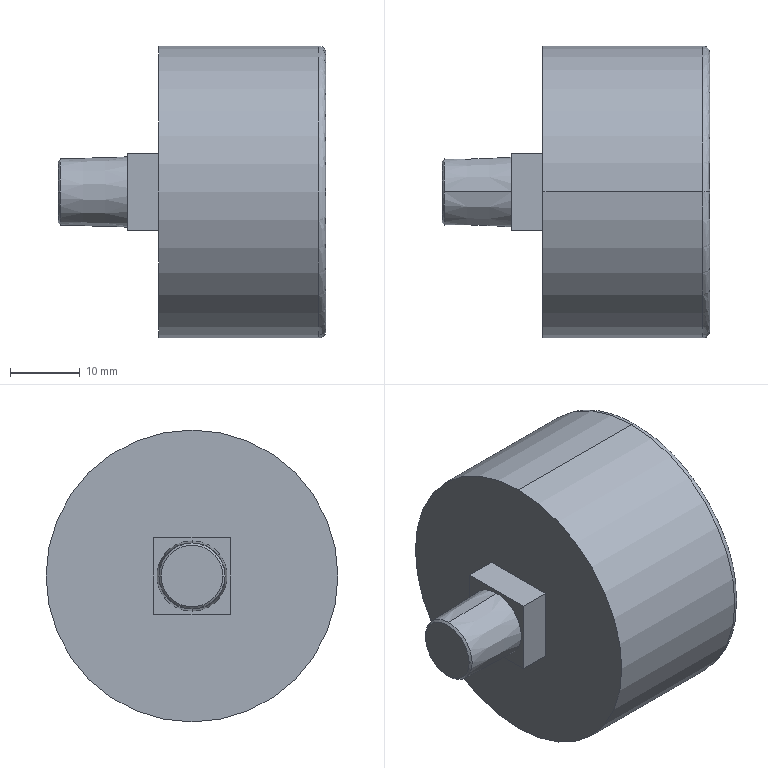Part | STEP file | 1 solid | 18 faces | box 38.5 x 42 x 42 mm | volume 33324 mm3 | plane 8 | cone 6 | cylinder 2 | spline 2 | commonest cylinder face diameters 42 x2
STEP:
#1=CARTESIAN_POINT('',(0.,0.,0.));
#2=DIRECTION('',(0.,0.,1.));
#3=DIRECTION('',(1.,0.,0.));
#4=AXIS2_PLACEMENT_3D('',#1,#2,#3);
#5=CARTESIAN_POINT('',(-38.2,0.,4.748));
#6=VERTEX_POINT('',#5);
#7=CARTESIAN_POINT('',(-38.2,4.748,0.));
#8=VERTEX_POINT('',#7);
#9=CARTESIAN_POINT('',(-38.2,0.,0.));
#10=DIRECTION('',(-1.,0.,0.));
#11=DIRECTION('',(0.,0.,-1.));
#12=AXIS2_PLACEMENT_3D('',#9,#10,#11);
#13=CIRCLE('',#12,4.748);
#14=CARTESIAN_POINT('',(-38.2,0.,0.));
#15=DIRECTION('',(1.,0.,0.));
#16=DIRECTION('',(0.,0.,-1.));
#17=AXIS2_PLACEMENT_3D('',#14,#15,#16);
#18=CONICAL_SURFACE('',#17,4.748,0.03121);
#19=CARTESIAN_POINT('',(6.283,0.));
#20=DIRECTION('',(-1.,0.));
#21=VECTOR('',#20,1.);
#22=LINE('',#19,#21);
#23=(GEOMETRIC_REPRESENTATION_CONTEXT(2)PARAMETRIC_REPRESENTATION_CONTEXT()REPRESENTATION_CONTEXT('',''));
#24=DEFINITIONAL_REPRESENTATION('',(#22),#23);
#25=PCURVE('',#18,#24);
#26=CARTESIAN_POINT('',(-38.5,0.,0.));
#27=DIRECTION('',(1.,0.,0.));
#28=DIRECTION('',(0.,1.,0.));
#29=AXIS2_PLACEMENT_3D('',#26,#27,#28);
#30=CONICAL_SURFACE('',#29,4.439,0.801);
#31=CARTESIAN_POINT('',(4.712,0.2999));
#32=DIRECTION('',(-1.,0.));
#33=VECTOR('',#32,1.);
#34=LINE('',#31,#33);
#35=(GEOMETRIC_REPRESENTATION_CONTEXT(2)PARAMETRIC_REPRESENTATION_CONTEXT()REPRESENTATION_CONTEXT('',''));
#36=DEFINITIONAL_REPRESENTATION('',(#34),#35);
#37=PCURVE('',#30,#36);
#38=SURFACE_CURVE('',#13,(#25,#37),.PCURVE_S1.);
#39=EDGE_CURVE('',#6,#8,#38,.T.);
#40=ORIENTED_EDGE('',*,*,#39,.F.);
#41=CARTESIAN_POINT('',(-28.5,0.,5.051));
#42=VERTEX_POINT('',#41);
#43=CARTESIAN_POINT('',(-38.2,0.,4.748));
#44=DIRECTION('',(0.9995,0.,0.0312));
#45=VECTOR('',#44,1.);
#46=LINE('',#43,#45);
#47=CARTESIAN_POINT('',(3.142,0.));
#48=DIRECTION('',(0.,1.));
#49=VECTOR('',#48,1.);
#50=LINE('',#47,#49);
#51=(GEOMETRIC_REPRESENTATION_CONTEXT(2)PARAMETRIC_REPRESENTATION_CONTEXT()REPRESENTATION_CONTEXT('',''));
#52=DEFINITIONAL_REPRESENTATION('',(#50),#51);
#53=PCURVE('',#18,#52);
#54=CARTESIAN_POINT('',(-38.2,0.,0.));
#55=DIRECTION('',(1.,0.,0.));
#56=DIRECTION('',(0.,0.,-1.));
#57=AXIS2_PLACEMENT_3D('',#54,#55,#56);
#58=CONICAL_SURFACE('',#57,4.748,0.03121);
#59=CARTESIAN_POINT('',(3.142,0.));
#60=DIRECTION('',(0.,1.));
#61=VECTOR('',#60,1.);
#62=LINE('',#59,#61);
#63=(GEOMETRIC_REPRESENTATION_CONTEXT(2)PARAMETRIC_REPRESENTATION_CONTEXT()REPRESENTATION_CONTEXT('',''));
#64=DEFINITIONAL_REPRESENTATION('',(#62),#63);
#65=PCURVE('',#58,#64);
#66=SURFACE_CURVE('',#46,(#53,#65),.PCURVE_S1.);
#67=EDGE_CURVE('',#6,#42,#66,.T.);
#68=ORIENTED_EDGE('',*,*,#67,.T.);
#69=CARTESIAN_POINT('',(-28.5,0.,-5.051));
#70=VERTEX_POINT('',#69);
#71=CARTESIAN_POINT('',(-28.5,0.,0.));
#72=DIRECTION('',(1.,0.,0.));
#73=DIRECTION('',(0.,0.,-1.));
#74=AXIS2_PLACEMENT_3D('',#71,#72,#73);
#75=CIRCLE('',#74,5.051);
#76=CARTESIAN_POINT('',(0.,9.7));
#77=DIRECTION('',(1.,0.));
#78=VECTOR('',#77,1.);
#79=LINE('',#76,#78);
#80=(GEOMETRIC_REPRESENTATION_CONTEXT(2)PARAMETRIC_REPRESENTATION_CONTEXT()REPRESENTATION_CONTEXT('',''));
#81=DEFINITIONAL_REPRESENTATION('',(#79),#80);
#82=PCURVE('',#18,#81);
#83=CARTESIAN_POINT('',(-28.5,-5.5,5.5));
#84=DIRECTION('',(1.,0.,0.));
#85=DIRECTION('',(0.,0.,-1.));
#86=AXIS2_PLACEMENT_3D('',#83,#84,#85);
#87=PLANE('',#86);
#88=CARTESIAN_POINT('',(5.5,5.5));
#89=DIRECTION('',(1.,0.));
#90=AXIS2_PLACEMENT_2D('',#88,#89);
#91=CIRCLE('',#90,5.051);
#92=(GEOMETRIC_REPRESENTATION_CONTEXT(2)PARAMETRIC_REPRESENTATION_CONTEXT()REPRESENTATION_CONTEXT('',''));
#93=DEFINITIONAL_REPRESENTATION('',(#91),#92);
#94=PCURVE('',#87,#93);
#95=SURFACE_CURVE('',#75,(#82,#94),.PCURVE_S1.);
#96=EDGE_CURVE('',#70,#42,#95,.T.);
#97=ORIENTED_EDGE('',*,*,#96,.F.);
#98=CARTESIAN_POINT('',(-38.2,0.,-4.748));
#99=VERTEX_POINT('',#98);
#100=CARTESIAN_POINT('',(-38.2,0.,-4.748));
#101=DIRECTION('',(0.9995,0.,-0.0312));
#102=VECTOR('',#101,1.);
#103=LINE('',#100,#102);
#104=CARTESIAN_POINT('',(0.,0.));
#105=DIRECTION('',(0.,1.));
#106=VECTOR('',#105,1.);
#107=LINE('',#104,#106);
#108=(GEOMETRIC_REPRESENTATION_CONTEXT(2)PARAMETRIC_REPRESENTATION_CONTEXT()REPRESENTATION_CONTEXT('',''));
#109=DEFINITIONAL_REPRESENTATION('',(#107),#108);
#110=PCURVE('',#18,#109);
#111=CARTESIAN_POINT('',(6.283,0.));
#112=DIRECTION('',(0.,1.));
#113=VECTOR('',#112,1.);
#114=LINE('',#111,#113);
#115=(GEOMETRIC_REPRESENTATION_CONTEXT(2)PARAMETRIC_REPRESENTATION_CONTEXT()REPRESENTATION_CONTEXT('',''));
#116=DEFINITIONAL_REPRESENTATION('',(#114),#115);
#117=PCURVE('',#58,#116);
#118=SURFACE_CURVE('',#103,(#110,#117),.PCURVE_S1.);
#119=EDGE_CURVE('',#99,#70,#118,.T.);
#120=ORIENTED_EDGE('',*,*,#119,.F.);
#121=CARTESIAN_POINT('',(-38.2,0.,0.));
#122=DIRECTION('',(-1.,0.,0.));
#123=DIRECTION('',(0.,0.,-1.));
#124=AXIS2_PLACEMENT_3D('',#121,#122,#123);
#125=CIRCLE('',#124,4.748);
#126=CARTESIAN_POINT('',(6.283,0.));
#127=DIRECTION('',(-1.,0.));
#128=VECTOR('',#127,1.);
#129=LINE('',#126,#128);
#130=(GEOMETRIC_REPRESENTATION_CONTEXT(2)PARAMETRIC_REPRESENTATION_CONTEXT()REPRESENTATION_CONTEXT('',''));
#131=DEFINITIONAL_REPRESENTATION('',(#129),#130);
#132=PCURVE('',#18,#131);
#133=CARTESIAN_POINT('',(-38.5,0.,0.));
#134=DIRECTION('',(1.,0.,0.));
#135=DIRECTION('',(0.,1.,0.));
#136=AXIS2_PLACEMENT_3D('',#133,#134,#135);
#137=CONICAL_SURFACE('',#136,4.439,0.801);
#138=CARTESIAN_POINT('',(10.996,0.2999));
#139=DIRECTION('',(-1.,0.));
#140=VECTOR('',#139,1.);
#141=LINE('',#138,#140);
#142=(GEOMETRIC_REPRESENTATION_CONTEXT(2)PARAMETRIC_REPRESENTATION_CONTEXT()REPRESENTATION_CONTEXT('',''));
#143=DEFINITIONAL_REPRESENTATION('',(#141),#142);
#144=PCURVE('',#137,#143);
#145=SURFACE_CURVE('',#125,(#132,#144),.PCURVE_S1.);
#146=EDGE_CURVE('',#8,#99,#145,.T.);
#147=ORIENTED_EDGE('',*,*,#146,.F.);
#148=EDGE_LOOP('',(#40,#68,#97,#120,#147));
#149=FACE_BOUND('',#148,.T.);
#150=ADVANCED_FACE('',(#149),#18,.T.);
#151=CARTESIAN_POINT('',(-38.5,-4.439,0.));
#152=VERTEX_POINT('',#151);
#153=CARTESIAN_POINT('',(-38.5,4.439,0.));
#154=VERTEX_POINT('',#153);
#155=CARTESIAN_POINT('',(-38.5,0.,0.));
#156=DIRECTION('',(-1.,0.,0.));
#157=DIRECTION('',(0.,1.,0.));
#158=AXIS2_PLACEMENT_3D('',#155,#156,#157);
#159=CIRCLE('',#158,4.439);
#160=CARTESIAN_POINT('',(6.283,0.));
#161=DIRECTION('',(-1.,0.));
#162=VECTOR('',#161,1.);
#163=LINE('',#160,#162);
#164=(GEOMETRIC_REPRESENTATION_CONTEXT(2)PARAMETRIC_REPRESENTATION_CONTEXT()REPRESENTATION_CONTEXT('',''));
#165=DEFINITIONAL_REPRESENTATION('',(#163),#164);
#166=PCURVE('',#30,#165);
#167=CARTESIAN_POINT('',(-38.5,-4.492,4.492));
#168=DIRECTION('',(1.,0.,0.));
#169=DIRECTION('',(0.,0.,-1.));
#170=AXIS2_PLACEMENT_3D('',#167,#168,#169);
#171=PLANE('',#170);
#172=CARTESIAN_POINT('',(4.492,8.932));
#173=CARTESIAN_POINT('',(12.181,8.932));
#174=CARTESIAN_POINT('',(8.337,2.273));
#175=CARTESIAN_POINT('',(4.492,-4.386));
#176=CARTESIAN_POINT('',(0.648,2.273));
#177=CARTESIAN_POINT('',(-3.196,8.932));
#178=CARTESIAN_POINT('',(4.492,8.932));
#179=(BOUNDED_CURVE()B_SPLINE_CURVE(2,(#172,#173,#174,#175,#176,#177,#178),.UNSPECIFIED.,.T.,.F.)B_SPLINE_CURVE_WITH_KNOTS((1,2,2,2,2,1),(-2.094,0.,2.094,4.189,6.283,8.378),.UNSPECIFIED.)CURVE()GEOMETRIC_REPRESENTATION_ITEM()RATIONAL_B_SPLINE_CURVE((1.,0.5,1.,0.5,1.,0.5,1.))REPRESENTATION_ITEM(''));
#180=(GEOMETRIC_REPRESENTATION_CONTEXT(2)PARAMETRIC_REPRESENTATION_CONTEXT()REPRESENTATION_CONTEXT('',''));
#181=DEFINITIONAL_REPRESENTATION('',(#179),#180);
#182=PCURVE('',#171,#181);
#183=SURFACE_CURVE('',#159,(#166,#182),.PCURVE_S1.);
#184=EDGE_CURVE('',#152,#154,#183,.T.);
#185=ORIENTED_EDGE('',*,*,#184,.F.);
#186=CARTESIAN_POINT('',(-38.2,-4.748,0.));
#187=VERTEX_POINT('',#186);
#188=CARTESIAN_POINT('',(-38.5,-4.439,0.));
#189=DIRECTION('',(0.696,-0.7181,0.));
#190=VECTOR('',#189,1.);
#191=LINE('',#188,#190);
#192=CARTESIAN_POINT('',(3.142,0.));
#193=DIRECTION('',(0.,1.));
#194=VECTOR('',#193,1.);
#195=LINE('',#192,#194);
#196=(GEOMETRIC_REPRESENTATION_CONTEXT(2)PARAMETRIC_REPRESENTATION_CONTEXT()REPRESENTATION_CONTEXT('',''));
#197=DEFINITIONAL_REPRESENTATION('',(#195),#196);
#198=PCURVE('',#30,#197);
#199=CARTESIAN_POINT('',(3.142,0.));
#200=DIRECTION('',(0.,1.));
#201=VECTOR('',#200,1.);
#202=LINE('',#199,#201);
#203=(GEOMETRIC_REPRESENTATION_CONTEXT(2)PARAMETRIC_REPRESENTATION_CONTEXT()REPRESENTATION_CONTEXT('',''));
#204=DEFINITIONAL_REPRESENTATION('',(#202),#203);
#205=PCURVE('',#137,#204);
#206=SURFACE_CURVE('',#191,(#198,#205),.PCURVE_S1.);
#207=EDGE_CURVE('',#152,#187,#206,.T.);
#208=ORIENTED_EDGE('',*,*,#207,.T.);
#209=CARTESIAN_POINT('',(-38.2,0.,0.));
#210=DIRECTION('',(-1.,0.,0.));
#211=DIRECTION('',(0.,0.,-1.));
#212=AXIS2_PLACEMENT_3D('',#209,#210,#211);
#213=CIRCLE('',#212,4.748);
#214=CARTESIAN_POINT('',(4.712,0.2999));
#215=DIRECTION('',(-1.,0.));
#216=VECTOR('',#215,1.);
#217=LINE('',#214,#216);
#218=(GEOMETRIC_REPRESENTATION_CONTEXT(2)PARAMETRIC_REPRESENTATION_CONTEXT()REPRESENTATION_CONTEXT('',''));
#219=DEFINITIONAL_REPRESENTATION('',(#217),#218);
#220=PCURVE('',#30,#219);
#221=CARTESIAN_POINT('',(6.283,0.));
#222=DIRECTION('',(-1.,0.));
#223=VECTOR('',#222,1.);
#224=LINE('',#221,#223);
#225=(GEOMETRIC_REPRESENTATION_CONTEXT(2)PARAMETRIC_REPRESENTATION_CONTEXT()REPRESENTATION_CONTEXT('',''));
#226=DEFINITIONAL_REPRESENTATION('',(#224),#225);
#227=PCURVE('',#58,#226);
#228=SURFACE_CURVE('',#213,(#220,#227),.PCURVE_S1.);
#229=EDGE_CURVE('',#187,#6,#228,.T.);
#230=ORIENTED_EDGE('',*,*,#229,.T.);
#231=ORIENTED_EDGE('',*,*,#39,.T.);
#232=CARTESIAN_POINT('',(-38.5,4.439,0.));
#233=DIRECTION('',(0.696,0.7181,0.));
#234=VECTOR('',#233,1.);
#235=LINE('',#232,#234);
#236=CARTESIAN_POINT('',(0.,0.));
#237=DIRECTION('',(0.,1.));
#238=VECTOR('',#237,1.);
#239=LINE('',#236,#238);
#240=(GEOMETRIC_REPRESENTATION_CONTEXT(2)PARAMETRIC_REPRESENTATION_CONTEXT()REPRESENTATION_CONTEXT('',''));
#241=DEFINITIONAL_REPRESENTATION('',(#239),#240);
#242=PCURVE('',#30,#241);
#243=CARTESIAN_POINT('',(6.283,0.));
#244=DIRECTION('',(0.,1.));
#245=VECTOR('',#244,1.);
#246=LINE('',#243,#245);
#247=(GEOMETRIC_REPRESENTATION_CONTEXT(2)PARAMETRIC_REPRESENTATION_CONTEXT()REPRESENTATION_CONTEXT('',''));
#248=DEFINITIONAL_REPRESENTATION('',(#246),#247);
#249=PCURVE('',#137,#248);
#250=SURFACE_CURVE('',#235,(#242,#249),.PCURVE_S1.);
#251=EDGE_CURVE('',#154,#8,#250,.T.);
#252=ORIENTED_EDGE('',*,*,#251,.F.);
#253=EDGE_LOOP('',(#185,#208,#230,#231,#252));
#254=FACE_BOUND('',#253,.T.);
#255=ADVANCED_FACE('',(#254),#30,.T.);
#256=CARTESIAN_POINT('',(-24.,0.,-21.));
#257=VERTEX_POINT('',#256);
#258=CARTESIAN_POINT('',(-24.,0.,21.));
#259=VERTEX_POINT('',#258);
#260=CARTESIAN_POINT('',(-24.,0.,0.));
#261=DIRECTION('',(1.,0.,0.));
#262=DIRECTION('',(0.,0.,-1.));
#263=AXIS2_PLACEMENT_3D('',#260,#261,#262);
#264=CIRCLE('',#263,21.);
#265=CARTESIAN_POINT('',(-24.,0.,0.));
#266=DIRECTION('',(1.,0.,0.));
#267=DIRECTION('',(0.,0.,-1.));
#268=AXIS2_PLACEMENT_3D('',#265,#266,#267);
#269=CYLINDRICAL_SURFACE('',#268,21.);
#270=CARTESIAN_POINT('',(0.,0.));
#271=DIRECTION('',(1.,0.));
#272=VECTOR('',#271,1.);
#273=LINE('',#270,#272);
#274=(GEOMETRIC_REPRESENTATION_CONTEXT(2)PARAMETRIC_REPRESENTATION_CONTEXT()REPRESENTATION_CONTEXT('',''));
#275=DEFINITIONAL_REPRESENTATION('',(#273),#274);
#276=PCURVE('',#269,#275);
#277=CARTESIAN_POINT('',(-24.,-21.252,21.252));
#278=DIRECTION('',(1.,0.,0.));
#279=DIRECTION('',(0.,0.,-1.));
#280=AXIS2_PLACEMENT_3D('',#277,#278,#279);
#281=PLANE('',#280);
#282=CARTESIAN_POINT('',(21.252,21.252));
#283=DIRECTION('',(1.,0.));
#284=AXIS2_PLACEMENT_2D('',#282,#283);
#285=CIRCLE('',#284,21.);
#286=(GEOMETRIC_REPRESENTATION_CONTEXT(2)PARAMETRIC_REPRESENTATION_CONTEXT()REPRESENTATION_CONTEXT('',''));
#287=DEFINITIONAL_REPRESENTATION('',(#285),#286);
#288=PCURVE('',#281,#287);
#289=SURFACE_CURVE('',#264,(#276,#288),.PCURVE_S1.);
#290=EDGE_CURVE('',#257,#259,#289,.T.);
#291=ORIENTED_EDGE('',*,*,#290,.T.);
#292=CARTESIAN_POINT('',(-1.,-0.000000006,21.));
#293=VERTEX_POINT('',#292);
#294=CARTESIAN_POINT('',(-24.,0.,21.));
#295=DIRECTION('',(1.,0.,0.));
#296=VECTOR('',#295,1.);
#297=LINE('',#294,#296);
#298=CARTESIAN_POINT('',(3.142,0.));
#299=DIRECTION('',(0.,1.));
#300=VECTOR('',#299,1.);
#301=LINE('',#298,#300);
#302=(GEOMETRIC_REPRESENTATION_CONTEXT(2)PARAMETRIC_REPRESENTATION_CONTEXT()REPRESENTATION_CONTEXT('',''));
#303=DEFINITIONAL_REPRESENTATION('',(#301),#302);
#304=PCURVE('',#269,#303);
#305=CARTESIAN_POINT('',(-24.,0.,0.));
#306=DIRECTION('',(1.,0.,0.));
#307=DIRECTION('',(0.,0.,-1.));
#308=AXIS2_PLACEMENT_3D('',#305,#306,#307);
#309=CYLINDRICAL_SURFACE('',#308,21.);
#310=CARTESIAN_POINT('',(3.142,0.));
#311=DIRECTION('',(0.,1.));
#312=VECTOR('',#311,1.);
#313=LINE('',#310,#312);
#314=(GEOMETRIC_REPRESENTATION_CONTEXT(2)PARAMETRIC_REPRESENTATION_CONTEXT()REPRESENTATION_CONTEXT('',''));
#315=DEFINITIONAL_REPRESENTATION('',(#313),#314);
#316=PCURVE('',#309,#315);
#317=SURFACE_CURVE('',#297,(#304,#316),.PCURVE_S1.);
#318=EDGE_CURVE('',#259,#293,#317,.T.);
#319=ORIENTED_EDGE('',*,*,#318,.T.);
#320=CARTESIAN_POINT('',(-1.,-0.000000001,-21.));
#321=VERTEX_POINT('',#320);
#322=CARTESIAN_POINT('',(-1.,0.,0.));
#323=DIRECTION('',(1.,0.,0.));
#324=DIRECTION('',(0.,0.,-1.));
#325=AXIS2_PLACEMENT_3D('',#322,#323,#324);
#326=CIRCLE('',#325,21.);
#327=CARTESIAN_POINT('',(0.,23.));
#328=DIRECTION('',(1.,0.));
#329=VECTOR('',#328,1.);
#330=LINE('',#327,#329);
#331=(GEOMETRIC_REPRESENTATION_CONTEXT(2)PARAMETRIC_REPRESENTATION_CONTEXT()REPRESENTATION_CONTEXT('',''));
#332=DEFINITIONAL_REPRESENTATION('',(#330),#331);
#333=PCURVE('',#269,#332);
#334=CARTESIAN_POINT('',(-0.004996,0.,-19.9));
#335=CARTESIAN_POINT('',(-0.004996,39.8,-19.9));
#336=CARTESIAN_POINT('',(-0.004996,39.8,19.9));
#337=CARTESIAN_POINT('',(-0.004996,0.,19.9));
#338=CARTESIAN_POINT('',(0.06322,0.,-20.58));
#339=CARTESIAN_POINT('',(0.06322,41.16,-20.58));
#340=CARTESIAN_POINT('',(0.06322,41.16,20.58));
#341=CARTESIAN_POINT('',(0.06322,0.,20.58));
#342=CARTESIAN_POINT('',(-0.4199,0.,-21.063));
#343=CARTESIAN_POINT('',(-0.4199,42.126,-21.063));
#344=CARTESIAN_POINT('',(-0.4199,42.126,21.063));
#345=CARTESIAN_POINT('',(-0.4199,0.,21.063));
#346=CARTESIAN_POINT('',(-1.1,0.,-20.995));
#347=CARTESIAN_POINT('',(-1.1,41.99,-20.995));
#348=CARTESIAN_POINT('',(-1.1,41.99,20.995));
#349=CARTESIAN_POINT('',(-1.1,0.,20.995));
#350=(BOUNDED_SURFACE()B_SPLINE_SURFACE(3,3,((#334,#335,#336,#337),(#338,#339,#340,#341),(#342,#343,#344,#345),(#346,#347,#348,#349)),.UNSPECIFIED.,.F.,.F.,.F.)B_SPLINE_SURFACE_WITH_KNOTS((4,4),(4,4),(0.,1.),(0.,1.),.PIECEWISE_BEZIER_KNOTS.)GEOMETRIC_REPRESENTATION_ITEM()RATIONAL_B_SPLINE_SURFACE(((1.,0.3333,0.3333,1.),(0.7553,0.2518,0.2518,0.7553),(0.7553,0.2518,0.2518,0.7553),(1.,0.3333,0.3333,1.)))REPRESENTATION_ITEM('')SURFACE());
#351=CARTESIAN_POINT('',(0.9369,0.));
#352=CARTESIAN_POINT('',(0.9369,0.02375));
#353=CARTESIAN_POINT('',(0.9369,0.06805));
#354=CARTESIAN_POINT('',(0.9369,0.1267));
#355=CARTESIAN_POINT('',(0.9369,0.1794));
#356=CARTESIAN_POINT('',(0.9369,0.2276));
#357=CARTESIAN_POINT('',(0.9369,0.2721));
#358=CARTESIAN_POINT('',(0.9369,0.3139));
#359=CARTESIAN_POINT('',(0.9369,0.3535));
#360=CARTESIAN_POINT('',(0.9369,0.3914));
#361=CARTESIAN_POINT('',(0.9369,0.4282));
#362=CARTESIAN_POINT('',(0.9369,0.4643));
#363=CARTESIAN_POINT('',(0.9369,0.5));
#364=CARTESIAN_POINT('',(0.9369,0.5357));
#365=CARTESIAN_POINT('',(0.9369,0.5718));
#366=CARTESIAN_POINT('',(0.9369,0.6086));
#367=CARTESIAN_POINT('',(0.9369,0.6465));
#368=CARTESIAN_POINT('',(0.9369,0.6861));
#369=CARTESIAN_POINT('',(0.9369,0.7279));
#370=CARTESIAN_POINT('',(0.9369,0.7724));
#371=CARTESIAN_POINT('',(0.9369,0.8206));
#372=CARTESIAN_POINT('',(0.9369,0.8733));
#373=CARTESIAN_POINT('',(0.9369,0.9319));
#374=CARTESIAN_POINT('',(0.9369,0.9763));
#375=CARTESIAN_POINT('',(0.9369,1.));
#376=B_SPLINE_CURVE_WITH_KNOTS('',3,(#351,#352,#353,#354,#355,#356,#357,#358,#359,#360,#361,#362,#363,#364,#365,#366,#367,#368,#369,#370,#371,#372,#373,#374,#375),.UNSPECIFIED.,.F.,.F.,(4,1,1,1,1,1,1,1,1,1,1,1,1,1,1,1,1,1,1,1,1,1,4),(0.,0.1428,0.2856,0.4284,0.5712,0.714,0.8568,0.9996,1.142,1.285,1.428,1.571,1.714,1.856,1.999,2.142,2.285,2.428,2.57,2.713,2.856,2.999,3.142),.QUASI_UNIFORM_KNOTS.);
#377=(GEOMETRIC_REPRESENTATION_CONTEXT(2)PARAMETRIC_REPRESENTATION_CONTEXT()REPRESENTATION_CONTEXT('',''));
#378=DEFINITIONAL_REPRESENTATION('',(#376),#377);
#379=PCURVE('',#350,#378);
#380=SURFACE_CURVE('',#326,(#333,#379),.PCURVE_S1.);
#381=EDGE_CURVE('',#321,#293,#380,.T.);
#382=ORIENTED_EDGE('',*,*,#381,.F.);
#383=CARTESIAN_POINT('',(-24.,0.,-21.));
#384=DIRECTION('',(1.,0.,0.));
#385=VECTOR('',#384,1.);
#386=LINE('',#383,#385);
#387=CARTESIAN_POINT('',(0.,0.));
#388=DIRECTION('',(0.,1.));
#389=VECTOR('',#388,1.);
#390=LINE('',#387,#389);
#391=(GEOMETRIC_REPRESENTATION_CONTEXT(2)PARAMETRIC_REPRESENTATION_CONTEXT()REPRESENTATION_CONTEXT('',''));
#392=DEFINITIONAL_REPRESENTATION('',(#390),#391);
#393=PCURVE('',#269,#392);
#394=CARTESIAN_POINT('',(6.283,0.));
#395=DIRECTION('',(0.,1.));
#396=VECTOR('',#395,1.);
#397=LINE('',#394,#396);
#398=(GEOMETRIC_REPRESENTATION_CONTEXT(2)PARAMETRIC_REPRESENTATION_CONTEXT()REPRESENTATION_CONTEXT('',''));
#399=DEFINITIONAL_REPRESENTATION('',(#397),#398);
#400=PCURVE('',#309,#399);
#401=SURFACE_CURVE('',#386,(#393,#400),.PCURVE_S1.);
#402=EDGE_CURVE('',#257,#321,#401,.T.);
#403=ORIENTED_EDGE('',*,*,#402,.F.);
#404=EDGE_LOOP('',(#291,#319,#382,#403));
#405=FACE_BOUND('',#404,.T.);
#406=ADVANCED_FACE('',(#405),#269,.T.);
#407=CARTESIAN_POINT('',(-1.,0.,-19.));
#408=VERTEX_POINT('',#407);
#409=CARTESIAN_POINT('',(0.,0.,-20.));
#410=VERTEX_POINT('',#409);
#411=CARTESIAN_POINT('',(-1.,0.,-19.));
#412=DIRECTION('',(0.7071,0.,-0.7071));
#413=VECTOR('',#412,1.);
#414=LINE('',#411,#413);
#415=CARTESIAN_POINT('',(-1.,0.,0.));
#416=DIRECTION('',(1.,0.,0.));
#417=DIRECTION('',(0.,0.,-1.));
#418=AXIS2_PLACEMENT_3D('',#415,#416,#417);
#419=CONICAL_SURFACE('',#418,19.,0.7854);
#420=CARTESIAN_POINT('',(6.283,0.));
#421=DIRECTION('',(0.,1.));
#422=VECTOR('',#421,1.);
#423=LINE('',#420,#422);
#424=(GEOMETRIC_REPRESENTATION_CONTEXT(2)PARAMETRIC_REPRESENTATION_CONTEXT()REPRESENTATION_CONTEXT('',''));
#425=DEFINITIONAL_REPRESENTATION('',(#423),#424);
#426=PCURVE('',#419,#425);
#427=CARTESIAN_POINT('',(-1.,0.,0.));
#428=DIRECTION('',(1.,0.,0.));
#429=DIRECTION('',(0.,0.,-1.));
#430=AXIS2_PLACEMENT_3D('',#427,#428,#429);
#431=CONICAL_SURFACE('',#430,19.,0.7854);
#432=CARTESIAN_POINT('',(0.,0.));
#433=DIRECTION('',(0.,1.));
#434=VECTOR('',#433,1.);
#435=LINE('',#432,#434);
#436=(GEOMETRIC_REPRESENTATION_CONTEXT(2)PARAMETRIC_REPRESENTATION_CONTEXT()REPRESENTATION_CONTEXT('',''));
#437=DEFINITIONAL_REPRESENTATION('',(#435),#436);
#438=PCURVE('',#431,#437);
#439=SURFACE_CURVE('',#414,(#426,#438),.PCURVE_S1.);
#440=EDGE_CURVE('',#408,#410,#439,.T.);
#441=ORIENTED_EDGE('',*,*,#440,.T.);
#442=CARTESIAN_POINT('',(0.,-0.000000002,20.));
#443=VERTEX_POINT('',#442);
#444=CARTESIAN_POINT('',(0.,0.,0.));
#445=DIRECTION('',(-1.,0.,0.));
#446=DIRECTION('',(0.,-1.,0.));
#447=AXIS2_PLACEMENT_3D('',#444,#445,#446);
#448=CIRCLE('',#447,20.);
#449=CARTESIAN_POINT('',(10.996,1.));
#450=DIRECTION('',(-1.,0.));
#451=VECTOR('',#450,1.);
#452=LINE('',#449,#451);
#453=(GEOMETRIC_REPRESENTATION_CONTEXT(2)PARAMETRIC_REPRESENTATION_CONTEXT()REPRESENTATION_CONTEXT('',''));
#454=DEFINITIONAL_REPRESENTATION('',(#452),#453);
#455=PCURVE('',#419,#454);
#456=CARTESIAN_POINT('',(-0.004996,0.,19.9));
#457=CARTESIAN_POINT('',(-0.004996,-39.8,19.9));
#458=CARTESIAN_POINT('',(-0.004996,-39.8,-19.9));
#459=CARTESIAN_POINT('',(-0.004996,0.,-19.9));
#460=CARTESIAN_POINT('',(0.06322,0.,20.58));
#461=CARTESIAN_POINT('',(0.06322,-41.16,20.58));
#462=CARTESIAN_POINT('',(0.06322,-41.16,-20.58));
#463=CARTESIAN_POINT('',(0.06322,0.,-20.58));
#464=CARTESIAN_POINT('',(-0.4199,0.,21.063));
#465=CARTESIAN_POINT('',(-0.4199,-42.126,21.063));
#466=CARTESIAN_POINT('',(-0.4199,-42.126,-21.063));
#467=CARTESIAN_POINT('',(-0.4199,0.,-21.063));
#468=CARTESIAN_POINT('',(-1.1,0.,20.995));
#469=CARTESIAN_POINT('',(-1.1,-41.99,20.995));
#470=CARTESIAN_POINT('',(-1.1,-41.99,-20.995));
#471=CARTESIAN_POINT('',(-1.1,0.,-20.995));
#472=(BOUNDED_SURFACE()B_SPLINE_SURFACE(3,3,((#456,#457,#458,#459),(#460,#461,#462,#463),(#464,#465,#466,#467),(#468,#469,#470,#471)),.UNSPECIFIED.,.F.,.F.,.F.)B_SPLINE_SURFACE_WITH_KNOTS((4,4),(4,4),(0.,1.),(0.,1.),.PIECEWISE_BEZIER_KNOTS.)GEOMETRIC_REPRESENTATION_ITEM()RATIONAL_B_SPLINE_SURFACE(((1.,0.3333,0.3333,1.),(0.7553,0.2518,0.2518,0.7553),(0.7553,0.2518,0.2518,0.7553),(1.,0.3333,0.3333,1.)))REPRESENTATION_ITEM('')SURFACE());
#473=CARTESIAN_POINT('',(0.06314,1.));
#474=CARTESIAN_POINT('',(0.06314,0.9763));
#475=CARTESIAN_POINT('',(0.06314,0.9319));
#476=CARTESIAN_POINT('',(0.06314,0.8733));
#477=CARTESIAN_POINT('',(0.06314,0.8206));
#478=CARTESIAN_POINT('',(0.06314,0.7724));
#479=CARTESIAN_POINT('',(0.06314,0.7279));
#480=CARTESIAN_POINT('',(0.06314,0.6861));
#481=CARTESIAN_POINT('',(0.06314,0.6465));
#482=CARTESIAN_POINT('',(0.06314,0.6086));
#483=CARTESIAN_POINT('',(0.06314,0.5718));
#484=CARTESIAN_POINT('',(0.06314,0.5357));
#485=CARTESIAN_POINT('',(0.06314,0.5));
#486=CARTESIAN_POINT('',(0.06314,0.4643));
#487=CARTESIAN_POINT('',(0.06314,0.4282));
#488=CARTESIAN_POINT('',(0.06314,0.3914));
#489=CARTESIAN_POINT('',(0.06314,0.3535));
#490=CARTESIAN_POINT('',(0.06314,0.3139));
#491=CARTESIAN_POINT('',(0.06314,0.2721));
#492=CARTESIAN_POINT('',(0.06314,0.2276));
#493=CARTESIAN_POINT('',(0.06314,0.1794));
#494=CARTESIAN_POINT('',(0.06314,0.1267));
#495=CARTESIAN_POINT('',(0.06314,0.06805));
#496=CARTESIAN_POINT('',(0.06314,0.02375));
#497=CARTESIAN_POINT('',(0.06314,0.));
#498=B_SPLINE_CURVE_WITH_KNOTS('',3,(#473,#474,#475,#476,#477,#478,#479,#480,#481,#482,#483,#484,#485,#486,#487,#488,#489,#490,#491,#492,#493,#494,#495,#496,#497),.UNSPECIFIED.,.F.,.F.,(4,1,1,1,1,1,1,1,1,1,1,1,1,1,1,1,1,1,1,1,1,1,4),(4.712,4.855,4.998,5.141,5.284,5.426,5.569,5.712,5.855,5.998,6.14,6.283,6.426,6.569,6.712,6.854,6.997,7.14,7.283,7.426,7.568,7.711,7.854),.QUASI_UNIFORM_KNOTS.);
#499=(GEOMETRIC_REPRESENTATION_CONTEXT(2)PARAMETRIC_REPRESENTATION_CONTEXT()REPRESENTATION_CONTEXT('',''));
#500=DEFINITIONAL_REPRESENTATION('',(#498),#499);
#501=PCURVE('',#472,#500);
#502=SURFACE_CURVE('',#448,(#455,#501),.PCURVE_S1.);
#503=EDGE_CURVE('',#410,#443,#502,.T.);
#504=ORIENTED_EDGE('',*,*,#503,.T.);
#505=CARTESIAN_POINT('',(-1.,0.,19.));
#506=VERTEX_POINT('',#505);
#507=CARTESIAN_POINT('',(-1.,0.,19.));
#508=DIRECTION('',(0.7071,0.,0.7071));
#509=VECTOR('',#508,1.);
#510=LINE('',#507,#509);
#511=CARTESIAN_POINT('',(3.142,0.));
#512=DIRECTION('',(0.,1.));
#513=VECTOR('',#512,1.);
#514=LINE('',#511,#513);
#515=(GEOMETRIC_REPRESENTATION_CONTEXT(2)PARAMETRIC_REPRESENTATION_CONTEXT()REPRESENTATION_CONTEXT('',''));
#516=DEFINITIONAL_REPRESENTATION('',(#514),#515);
#517=PCURVE('',#419,#516);
#518=CARTESIAN_POINT('',(3.142,0.));
#519=DIRECTION('',(0.,1.));
#520=VECTOR('',#519,1.);
#521=LINE('',#518,#520);
#522=(GEOMETRIC_REPRESENTATION_CONTEXT(2)PARAMETRIC_REPRESENTATION_CONTEXT()REPRESENTATION_CONTEXT('',''));
#523=DEFINITIONAL_REPRESENTATION('',(#521),#522);
#524=PCURVE('',#431,#523);
#525=SURFACE_CURVE('',#510,(#517,#524),.PCURVE_S1.);
#526=EDGE_CURVE('',#506,#443,#525,.T.);
#527=ORIENTED_EDGE('',*,*,#526,.F.);
#528=CARTESIAN_POINT('',(-1.,0.,0.));
#529=DIRECTION('',(-1.,0.,0.));
#530=DIRECTION('',(0.,0.,-1.));
#531=AXIS2_PLACEMENT_3D('',#528,#529,#530);
#532=CIRCLE('',#531,19.);
#533=CARTESIAN_POINT('',(6.283,0.));
#534=DIRECTION('',(-1.,0.));
#535=VECTOR('',#534,1.);
#536=LINE('',#533,#535);
#537=(GEOMETRIC_REPRESENTATION_CONTEXT(2)PARAMETRIC_REPRESENTATION_CONTEXT()REPRESENTATION_CONTEXT('',''));
#538=DEFINITIONAL_REPRESENTATION('',(#536),#537);
#539=PCURVE('',#419,#538);
#540=CARTESIAN_POINT('',(-1.,-19.228,-19.228));
#541=DIRECTION('',(-1.,0.,0.));
#542=DIRECTION('',(0.,0.,1.));
#543=AXIS2_PLACEMENT_3D('',#540,#541,#542);
#544=PLANE('',#543);
#545=CARTESIAN_POINT('',(19.228,19.228));
#546=DIRECTION('',(-1.,0.));
#547=AXIS2_PLACEMENT_2D('',#545,#546);
#548=CIRCLE('',#547,19.);
#549=(GEOMETRIC_REPRESENTATION_CONTEXT(2)PARAMETRIC_REPRESENTATION_CONTEXT()REPRESENTATION_CONTEXT('',''));
#550=DEFINITIONAL_REPRESENTATION('',(#548),#549);
#551=PCURVE('',#544,#550);
#552=SURFACE_CURVE('',#532,(#539,#551),.PCURVE_S1.);
#553=EDGE_CURVE('',#408,#506,#552,.T.);
#554=ORIENTED_EDGE('',*,*,#553,.F.);
#555=EDGE_LOOP('',(#441,#504,#527,#554));
#556=FACE_BOUND('',#555,.F.);
#557=ADVANCED_FACE('',(#556),#419,.F.);
#558=ORIENTED_EDGE('',*,*,#67,.F.);
#559=ORIENTED_EDGE('',*,*,#229,.F.);
#560=CARTESIAN_POINT('',(-38.2,0.,0.));
#561=DIRECTION('',(-1.,0.,0.));
#562=DIRECTION('',(0.,0.,-1.));
#563=AXIS2_PLACEMENT_3D('',#560,#561,#562);
#564=CIRCLE('',#563,4.748);
#565=CARTESIAN_POINT('',(6.283,0.));
#566=DIRECTION('',(-1.,0.));
#567=VECTOR('',#566,1.);
#568=LINE('',#565,#567);
#569=(GEOMETRIC_REPRESENTATION_CONTEXT(2)PARAMETRIC_REPRESENTATION_CONTEXT()REPRESENTATION_CONTEXT('',''));
#570=DEFINITIONAL_REPRESENTATION('',(#568),#569);
#571=PCURVE('',#58,#570);
#572=CARTESIAN_POINT('',(4.712,0.2999));
#573=DIRECTION('',(-1.,0.));
#574=VECTOR('',#573,1.);
#575=LINE('',#572,#574);
#576=(GEOMETRIC_REPRESENTATION_CONTEXT(2)PARAMETRIC_REPRESENTATION_CONTEXT()REPRESENTATION_CONTEXT('',''));
#577=DEFINITIONAL_REPRESENTATION('',(#575),#576);
#578=PCURVE('',#137,#577);
#579=SURFACE_CURVE('',#564,(#571,#578),.PCURVE_S1.);
#580=EDGE_CURVE('',#99,#187,#579,.T.);
#581=ORIENTED_EDGE('',*,*,#580,.F.);
#582=ORIENTED_EDGE('',*,*,#119,.T.);
#583=CARTESIAN_POINT('',(-28.5,0.,0.));
#584=DIRECTION('',(1.,0.,0.));
#585=DIRECTION('',(0.,0.,-1.));
#586=AXIS2_PLACEMENT_3D('',#583,#584,#585);
#587=CIRCLE('',#586,5.051);
#588=CARTESIAN_POINT('',(0.,9.7));
#589=DIRECTION('',(1.,0.));
#590=VECTOR('',#589,1.);
#591=LINE('',#588,#590);
#592=(GEOMETRIC_REPRESENTATION_CONTEXT(2)PARAMETRIC_REPRESENTATION_CONTEXT()REPRESENTATION_CONTEXT('',''));
#593=DEFINITIONAL_REPRESENTATION('',(#591),#592);
#594=PCURVE('',#58,#593);
#595=CARTESIAN_POINT('',(5.5,5.5));
#596=DIRECTION('',(1.,0.));
#597=AXIS2_PLACEMENT_2D('',#595,#596);
#598=CIRCLE('',#597,5.051);
#599=(GEOMETRIC_REPRESENTATION_CONTEXT(2)PARAMETRIC_REPRESENTATION_CONTEXT()REPRESENTATION_CONTEXT('',''));
#600=DEFINITIONAL_REPRESENTATION('',(#598),#599);
#601=PCURVE('',#87,#600);
#602=SURFACE_CURVE('',#587,(#594,#601),.PCURVE_S1.);
#603=EDGE_CURVE('',#42,#70,#602,.T.);
#604=ORIENTED_EDGE('',*,*,#603,.F.);
#605=EDGE_LOOP('',(#558,#559,#581,#582,#604));
#606=FACE_BOUND('',#605,.T.);
#607=ADVANCED_FACE('',(#606),#58,.T.);
#608=ORIENTED_EDGE('',*,*,#207,.F.);
#609=CARTESIAN_POINT('',(-38.5,0.,0.));
#610=DIRECTION('',(-1.,0.,0.));
#611=DIRECTION('',(0.,1.,0.));
#612=AXIS2_PLACEMENT_3D('',#609,#610,#611);
#613=CIRCLE('',#612,4.439);
#614=CARTESIAN_POINT('',(6.283,0.));
#615=DIRECTION('',(-1.,0.));
#616=VECTOR('',#615,1.);
#617=LINE('',#614,#616);
#618=(GEOMETRIC_REPRESENTATION_CONTEXT(2)PARAMETRIC_REPRESENTATION_CONTEXT()REPRESENTATION_CONTEXT('',''));
#619=DEFINITIONAL_REPRESENTATION('',(#617),#618);
#620=PCURVE('',#137,#619);
#621=CARTESIAN_POINT('',(4.492,8.932));
#622=CARTESIAN_POINT('',(12.181,8.932));
#623=CARTESIAN_POINT('',(8.337,2.273));
#624=CARTESIAN_POINT('',(4.492,-4.386));
#625=CARTESIAN_POINT('',(0.648,2.273));
#626=CARTESIAN_POINT('',(-3.196,8.932));
#627=CARTESIAN_POINT('',(4.492,8.932));
#628=(BOUNDED_CURVE()B_SPLINE_CURVE(2,(#621,#622,#623,#624,#625,#626,#627),.UNSPECIFIED.,.T.,.F.)B_SPLINE_CURVE_WITH_KNOTS((1,2,2,2,2,1),(-2.094,0.,2.094,4.189,6.283,8.378),.UNSPECIFIED.)CURVE()GEOMETRIC_REPRESENTATION_ITEM()RATIONAL_B_SPLINE_CURVE((1.,0.5,1.,0.5,1.,0.5,1.))REPRESENTATION_ITEM(''));
#629=(GEOMETRIC_REPRESENTATION_CONTEXT(2)PARAMETRIC_REPRESENTATION_CONTEXT()REPRESENTATION_CONTEXT('',''));
#630=DEFINITIONAL_REPRESENTATION('',(#628),#629);
#631=PCURVE('',#171,#630);
#632=SURFACE_CURVE('',#613,(#620,#631),.PCURVE_S1.);
#633=EDGE_CURVE('',#154,#152,#632,.T.);
#634=ORIENTED_EDGE('',*,*,#633,.F.);
#635=ORIENTED_EDGE('',*,*,#251,.T.);
#636=ORIENTED_EDGE('',*,*,#146,.T.);
#637=ORIENTED_EDGE('',*,*,#580,.T.);
#638=EDGE_LOOP('',(#608,#634,#635,#636,#637));
#639=FACE_BOUND('',#638,.T.);
#640=ADVANCED_FACE('',(#639),#137,.T.);
#641=ORIENTED_EDGE('',*,*,#96,.T.);
#642=ORIENTED_EDGE('',*,*,#603,.T.);
#643=EDGE_LOOP('',(#641,#642));
#644=FACE_BOUND('',#643,.T.);
#645=CARTESIAN_POINT('',(-28.5,-5.5,-5.5));
#646=VERTEX_POINT('',#645);
#647=CARTESIAN_POINT('',(-28.5,5.5,-5.5));
#648=VERTEX_POINT('',#647);
#649=CARTESIAN_POINT('',(-28.5,0.,-5.5));
#650=DIRECTION('',(0.,1.,0.));
#651=VECTOR('',#650,1.);
#652=LINE('',#649,#651);
#653=CARTESIAN_POINT('',(11.,5.5));
#654=DIRECTION('',(0.,1.));
#655=VECTOR('',#654,1.);
#656=LINE('',#653,#655);
#657=(GEOMETRIC_REPRESENTATION_CONTEXT(2)PARAMETRIC_REPRESENTATION_CONTEXT()REPRESENTATION_CONTEXT('',''));
#658=DEFINITIONAL_REPRESENTATION('',(#656),#657);
#659=PCURVE('',#87,#658);
#660=CARTESIAN_POINT('',(-24.,-5.5,-5.5));
#661=DIRECTION('',(0.,0.,-1.));
#662=DIRECTION('',(-1.,0.,0.));
#663=AXIS2_PLACEMENT_3D('',#660,#661,#662);
#664=PLANE('',#663);
#665=CARTESIAN_POINT('',(4.5,5.5));
#666=DIRECTION('',(0.,1.));
#667=VECTOR('',#666,1.);
#668=LINE('',#665,#667);
#669=(GEOMETRIC_REPRESENTATION_CONTEXT(2)PARAMETRIC_REPRESENTATION_CONTEXT()REPRESENTATION_CONTEXT('',''));
#670=DEFINITIONAL_REPRESENTATION('',(#668),#669);
#671=PCURVE('',#664,#670);
#672=SURFACE_CURVE('',#652,(#659,#671),.PCURVE_S1.);
#673=EDGE_CURVE('',#646,#648,#672,.T.);
#674=ORIENTED_EDGE('',*,*,#673,.F.);
#675=CARTESIAN_POINT('',(-28.5,-5.5,5.5));
#676=VERTEX_POINT('',#675);
#677=CARTESIAN_POINT('',(-28.5,-5.5,0.));
#678=DIRECTION('',(0.,0.,-1.));
#679=VECTOR('',#678,1.);
#680=LINE('',#677,#679);
#681=CARTESIAN_POINT('',(5.5,0.));
#682=DIRECTION('',(1.,0.));
#683=VECTOR('',#682,1.);
#684=LINE('',#681,#683);
#685=(GEOMETRIC_REPRESENTATION_CONTEXT(2)PARAMETRIC_REPRESENTATION_CONTEXT()REPRESENTATION_CONTEXT('',''));
#686=DEFINITIONAL_REPRESENTATION('',(#684),#685);
#687=PCURVE('',#87,#686);
#688=CARTESIAN_POINT('',(-28.5,-5.5,5.5));
#689=DIRECTION('',(0.,-1.,0.));
#690=DIRECTION('',(0.,0.,-1.));
#691=AXIS2_PLACEMENT_3D('',#688,#689,#690);
#692=PLANE('',#691);
#693=CARTESIAN_POINT('',(5.5,0.));
#694=DIRECTION('',(1.,0.));
#695=VECTOR('',#694,1.);
#696=LINE('',#693,#695);
#697=(GEOMETRIC_REPRESENTATION_CONTEXT(2)PARAMETRIC_REPRESENTATION_CONTEXT()REPRESENTATION_CONTEXT('',''));
#698=DEFINITIONAL_REPRESENTATION('',(#696),#697);
#699=PCURVE('',#692,#698);
#700=SURFACE_CURVE('',#680,(#687,#699),.PCURVE_S1.);
#701=EDGE_CURVE('',#676,#646,#700,.T.);
#702=ORIENTED_EDGE('',*,*,#701,.F.);
#703=CARTESIAN_POINT('',(-28.5,5.5,5.5));
#704=VERTEX_POINT('',#703);
#705=CARTESIAN_POINT('',(-28.5,0.,5.5));
#706=DIRECTION('',(0.,-1.,0.));
#707=VECTOR('',#706,1.);
#708=LINE('',#705,#707);
#709=CARTESIAN_POINT('',(0.,5.5));
#710=DIRECTION('',(0.,-1.));
#711=VECTOR('',#710,1.);
#712=LINE('',#709,#711);
#713=(GEOMETRIC_REPRESENTATION_CONTEXT(2)PARAMETRIC_REPRESENTATION_CONTEXT()REPRESENTATION_CONTEXT('',''));
#714=DEFINITIONAL_REPRESENTATION('',(#712),#713);
#715=PCURVE('',#87,#714);
#716=CARTESIAN_POINT('',(-28.5,-5.5,5.5));
#717=DIRECTION('',(0.,0.,1.));
#718=DIRECTION('',(1.,0.,0.));
#719=AXIS2_PLACEMENT_3D('',#716,#717,#718);
#720=PLANE('',#719);
#721=CARTESIAN_POINT('',(0.,5.5));
#722=DIRECTION('',(0.,-1.));
#723=VECTOR('',#722,1.);
#724=LINE('',#721,#723);
#725=(GEOMETRIC_REPRESENTATION_CONTEXT(2)PARAMETRIC_REPRESENTATION_CONTEXT()REPRESENTATION_CONTEXT('',''));
#726=DEFINITIONAL_REPRESENTATION('',(#724),#725);
#727=PCURVE('',#720,#726);
#728=SURFACE_CURVE('',#708,(#715,#727),.PCURVE_S1.);
#729=EDGE_CURVE('',#704,#676,#728,.T.);
#730=ORIENTED_EDGE('',*,*,#729,.F.);
#731=CARTESIAN_POINT('',(-28.5,5.5,0.));
#732=DIRECTION('',(0.,0.,1.));
#733=VECTOR('',#732,1.);
#734=LINE('',#731,#733);
#735=CARTESIAN_POINT('',(5.5,11.));
#736=DIRECTION('',(-1.,0.));
#737=VECTOR('',#736,1.);
#738=LINE('',#735,#737);
#739=(GEOMETRIC_REPRESENTATION_CONTEXT(2)PARAMETRIC_REPRESENTATION_CONTEXT()REPRESENTATION_CONTEXT('',''));
#740=DEFINITIONAL_REPRESENTATION('',(#738),#739);
#741=PCURVE('',#87,#740);
#742=CARTESIAN_POINT('',(-28.5,5.5,-5.5));
#743=DIRECTION('',(0.,1.,0.));
#744=DIRECTION('',(0.,0.,1.));
#745=AXIS2_PLACEMENT_3D('',#742,#743,#744);
#746=PLANE('',#745);
#747=CARTESIAN_POINT('',(5.5,0.));
#748=DIRECTION('',(1.,0.));
#749=VECTOR('',#748,1.);
#750=LINE('',#747,#749);
#751=(GEOMETRIC_REPRESENTATION_CONTEXT(2)PARAMETRIC_REPRESENTATION_CONTEXT()REPRESENTATION_CONTEXT('',''));
#752=DEFINITIONAL_REPRESENTATION('',(#750),#751);
#753=PCURVE('',#746,#752);
#754=SURFACE_CURVE('',#734,(#741,#753),.PCURVE_S1.);
#755=EDGE_CURVE('',#648,#704,#754,.T.);
#756=ORIENTED_EDGE('',*,*,#755,.F.);
#757=EDGE_LOOP('',(#674,#702,#730,#756));
#758=FACE_BOUND('',#757,.T.);
#759=ADVANCED_FACE('',(#644,#758),#87,.F.);
#760=ORIENTED_EDGE('',*,*,#633,.T.);
#761=ORIENTED_EDGE('',*,*,#184,.T.);
#762=EDGE_LOOP('',(#760,#761));
#763=FACE_BOUND('',#762,.T.);
#764=ADVANCED_FACE('',(#763),#171,.F.);
#765=CARTESIAN_POINT('',(-24.,5.5,5.5));
#766=VERTEX_POINT('',#765);
#767=CARTESIAN_POINT('',(-24.,5.5,-5.5));
#768=VERTEX_POINT('',#767);
#769=CARTESIAN_POINT('',(-24.,5.5,0.));
#770=DIRECTION('',(0.,0.,-1.));
#771=VECTOR('',#770,1.);
#772=LINE('',#769,#771);
#773=CARTESIAN_POINT('',(5.5,4.5));
#774=DIRECTION('',(-1.,0.));
#775=VECTOR('',#774,1.);
#776=LINE('',#773,#775);
#777=(GEOMETRIC_REPRESENTATION_CONTEXT(2)PARAMETRIC_REPRESENTATION_CONTEXT()REPRESENTATION_CONTEXT('',''));
#778=DEFINITIONAL_REPRESENTATION('',(#776),#777);
#779=PCURVE('',#746,#778);
#780=CARTESIAN_POINT('',(21.252,26.752));
#781=DIRECTION('',(1.,0.));
#782=VECTOR('',#781,1.);
#783=LINE('',#780,#782);
#784=(GEOMETRIC_REPRESENTATION_CONTEXT(2)PARAMETRIC_REPRESENTATION_CONTEXT()REPRESENTATION_CONTEXT('',''));
#785=DEFINITIONAL_REPRESENTATION('',(#783),#784);
#786=PCURVE('',#281,#785);
#787=SURFACE_CURVE('',#772,(#779,#786),.PCURVE_S1.);
#788=EDGE_CURVE('',#766,#768,#787,.T.);
#789=ORIENTED_EDGE('',*,*,#788,.T.);
#790=CARTESIAN_POINT('',(-26.25,5.5,-5.5));
#791=DIRECTION('',(-1.,0.,0.));
#792=VECTOR('',#791,1.);
#793=LINE('',#790,#792);
#794=CARTESIAN_POINT('',(0.,2.25));
#795=DIRECTION('',(0.,-1.));
#796=VECTOR('',#795,1.);
#797=LINE('',#794,#796);
#798=(GEOMETRIC_REPRESENTATION_CONTEXT(2)PARAMETRIC_REPRESENTATION_CONTEXT()REPRESENTATION_CONTEXT('',''));
#799=DEFINITIONAL_REPRESENTATION('',(#797),#798);
#800=PCURVE('',#746,#799);
#801=CARTESIAN_POINT('',(2.25,11.));
#802=DIRECTION('',(1.,0.));
#803=VECTOR('',#802,1.);
#804=LINE('',#801,#803);
#805=(GEOMETRIC_REPRESENTATION_CONTEXT(2)PARAMETRIC_REPRESENTATION_CONTEXT()REPRESENTATION_CONTEXT('',''));
#806=DEFINITIONAL_REPRESENTATION('',(#804),#805);
#807=PCURVE('',#664,#806);
#808=SURFACE_CURVE('',#793,(#800,#807),.PCURVE_S1.);
#809=EDGE_CURVE('',#768,#648,#808,.T.);
#810=ORIENTED_EDGE('',*,*,#809,.T.);
#811=ORIENTED_EDGE('',*,*,#755,.T.);
#812=CARTESIAN_POINT('',(-26.25,5.5,5.5));
#813=DIRECTION('',(1.,0.,0.));
#814=VECTOR('',#813,1.);
#815=LINE('',#812,#814);
#816=CARTESIAN_POINT('',(11.,2.25));
#817=DIRECTION('',(0.,1.));
#818=VECTOR('',#817,1.);
#819=LINE('',#816,#818);
#820=(GEOMETRIC_REPRESENTATION_CONTEXT(2)PARAMETRIC_REPRESENTATION_CONTEXT()REPRESENTATION_CONTEXT('',''));
#821=DEFINITIONAL_REPRESENTATION('',(#819),#820);
#822=PCURVE('',#746,#821);
#823=CARTESIAN_POINT('',(2.25,11.));
#824=DIRECTION('',(1.,0.));
#825=VECTOR('',#824,1.);
#826=LINE('',#823,#825);
#827=(GEOMETRIC_REPRESENTATION_CONTEXT(2)PARAMETRIC_REPRESENTATION_CONTEXT()REPRESENTATION_CONTEXT('',''));
#828=DEFINITIONAL_REPRESENTATION('',(#826),#827);
#829=PCURVE('',#720,#828);
#830=SURFACE_CURVE('',#815,(#822,#829),.PCURVE_S1.);
#831=EDGE_CURVE('',#704,#766,#830,.T.);
#832=ORIENTED_EDGE('',*,*,#831,.T.);
#833=EDGE_LOOP('',(#789,#810,#811,#832));
#834=FACE_BOUND('',#833,.T.);
#835=ADVANCED_FACE('',(#834),#746,.T.);
#836=CARTESIAN_POINT('',(-24.,-5.5,-5.5));
#837=VERTEX_POINT('',#836);
#838=CARTESIAN_POINT('',(-24.,0.,-5.5));
#839=DIRECTION('',(0.,-1.,0.));
#840=VECTOR('',#839,1.);
#841=LINE('',#838,#840);
#842=CARTESIAN_POINT('',(0.,5.5));
#843=DIRECTION('',(0.,-1.));
#844=VECTOR('',#843,1.);
#845=LINE('',#842,#844);
#846=(GEOMETRIC_REPRESENTATION_CONTEXT(2)PARAMETRIC_REPRESENTATION_CONTEXT()REPRESENTATION_CONTEXT('',''));
#847=DEFINITIONAL_REPRESENTATION('',(#845),#846);
#848=PCURVE('',#664,#847);
#849=CARTESIAN_POINT('',(26.752,21.252));
#850=DIRECTION('',(0.,-1.));
#851=VECTOR('',#850,1.);
#852=LINE('',#849,#851);
#853=(GEOMETRIC_REPRESENTATION_CONTEXT(2)PARAMETRIC_REPRESENTATION_CONTEXT()REPRESENTATION_CONTEXT('',''));
#854=DEFINITIONAL_REPRESENTATION('',(#852),#853);
#855=PCURVE('',#281,#854);
#856=SURFACE_CURVE('',#841,(#848,#855),.PCURVE_S1.);
#857=EDGE_CURVE('',#768,#837,#856,.T.);
#858=ORIENTED_EDGE('',*,*,#857,.T.);
#859=CARTESIAN_POINT('',(-26.25,-5.5,-5.5));
#860=DIRECTION('',(-1.,0.,0.));
#861=VECTOR('',#860,1.);
#862=LINE('',#859,#861);
#863=CARTESIAN_POINT('',(2.25,0.));
#864=DIRECTION('',(1.,0.));
#865=VECTOR('',#864,1.);
#866=LINE('',#863,#865);
#867=(GEOMETRIC_REPRESENTATION_CONTEXT(2)PARAMETRIC_REPRESENTATION_CONTEXT()REPRESENTATION_CONTEXT('',''));
#868=DEFINITIONAL_REPRESENTATION('',(#866),#867);
#869=PCURVE('',#664,#868);
#870=CARTESIAN_POINT('',(11.,2.25));
#871=DIRECTION('',(0.,-1.));
#872=VECTOR('',#871,1.);
#873=LINE('',#870,#872);
#874=(GEOMETRIC_REPRESENTATION_CONTEXT(2)PARAMETRIC_REPRESENTATION_CONTEXT()REPRESENTATION_CONTEXT('',''));
#875=DEFINITIONAL_REPRESENTATION('',(#873),#874);
#876=PCURVE('',#692,#875);
#877=SURFACE_CURVE('',#862,(#869,#876),.PCURVE_S1.);
#878=EDGE_CURVE('',#837,#646,#877,.T.);
#879=ORIENTED_EDGE('',*,*,#878,.T.);
#880=ORIENTED_EDGE('',*,*,#673,.T.);
#881=ORIENTED_EDGE('',*,*,#809,.F.);
#882=EDGE_LOOP('',(#858,#879,#880,#881));
#883=FACE_BOUND('',#882,.T.);
#884=ADVANCED_FACE('',(#883),#664,.T.);
#885=CARTESIAN_POINT('',(-24.,-5.5,5.5));
#886=VERTEX_POINT('',#885);
#887=CARTESIAN_POINT('',(-24.,-5.5,0.));
#888=DIRECTION('',(0.,0.,1.));
#889=VECTOR('',#888,1.);
#890=LINE('',#887,#889);
#891=CARTESIAN_POINT('',(5.5,4.5));
#892=DIRECTION('',(-1.,0.));
#893=VECTOR('',#892,1.);
#894=LINE('',#891,#893);
#895=(GEOMETRIC_REPRESENTATION_CONTEXT(2)PARAMETRIC_REPRESENTATION_CONTEXT()REPRESENTATION_CONTEXT('',''));
#896=DEFINITIONAL_REPRESENTATION('',(#894),#895);
#897=PCURVE('',#692,#896);
#898=CARTESIAN_POINT('',(21.252,15.752));
#899=DIRECTION('',(-1.,0.));
#900=VECTOR('',#899,1.);
#901=LINE('',#898,#900);
#902=(GEOMETRIC_REPRESENTATION_CONTEXT(2)PARAMETRIC_REPRESENTATION_CONTEXT()REPRESENTATION_CONTEXT('',''));
#903=DEFINITIONAL_REPRESENTATION('',(#901),#902);
#904=PCURVE('',#281,#903);
#905=SURFACE_CURVE('',#890,(#897,#904),.PCURVE_S1.);
#906=EDGE_CURVE('',#837,#886,#905,.T.);
#907=ORIENTED_EDGE('',*,*,#906,.T.);
#908=CARTESIAN_POINT('',(-26.25,-5.5,5.5));
#909=DIRECTION('',(-1.,0.,0.));
#910=VECTOR('',#909,1.);
#911=LINE('',#908,#910);
#912=CARTESIAN_POINT('',(0.,2.25));
#913=DIRECTION('',(0.,-1.));
#914=VECTOR('',#913,1.);
#915=LINE('',#912,#914);
#916=(GEOMETRIC_REPRESENTATION_CONTEXT(2)PARAMETRIC_REPRESENTATION_CONTEXT()REPRESENTATION_CONTEXT('',''));
#917=DEFINITIONAL_REPRESENTATION('',(#915),#916);
#918=PCURVE('',#692,#917);
#919=CARTESIAN_POINT('',(2.25,0.));
#920=DIRECTION('',(-1.,0.));
#921=VECTOR('',#920,1.);
#922=LINE('',#919,#921);
#923=(GEOMETRIC_REPRESENTATION_CONTEXT(2)PARAMETRIC_REPRESENTATION_CONTEXT()REPRESENTATION_CONTEXT('',''));
#924=DEFINITIONAL_REPRESENTATION('',(#922),#923);
#925=PCURVE('',#720,#924);
#926=SURFACE_CURVE('',#911,(#918,#925),.PCURVE_S1.);
#927=EDGE_CURVE('',#886,#676,#926,.T.);
#928=ORIENTED_EDGE('',*,*,#927,.T.);
#929=ORIENTED_EDGE('',*,*,#701,.T.);
#930=ORIENTED_EDGE('',*,*,#878,.F.);
#931=EDGE_LOOP('',(#907,#928,#929,#930));
#932=FACE_BOUND('',#931,.T.);
#933=ADVANCED_FACE('',(#932),#692,.T.);
#934=CARTESIAN_POINT('',(-24.,0.,5.5));
#935=DIRECTION('',(0.,1.,0.));
#936=VECTOR('',#935,1.);
#937=LINE('',#934,#936);
#938=CARTESIAN_POINT('',(4.5,5.5));
#939=DIRECTION('',(0.,1.));
#940=VECTOR('',#939,1.);
#941=LINE('',#938,#940);
#942=(GEOMETRIC_REPRESENTATION_CONTEXT(2)PARAMETRIC_REPRESENTATION_CONTEXT()REPRESENTATION_CONTEXT('',''));
#943=DEFINITIONAL_REPRESENTATION('',(#941),#942);
#944=PCURVE('',#720,#943);
#945=CARTESIAN_POINT('',(15.752,21.252));
#946=DIRECTION('',(0.,1.));
#947=VECTOR('',#946,1.);
#948=LINE('',#945,#947);
#949=(GEOMETRIC_REPRESENTATION_CONTEXT(2)PARAMETRIC_REPRESENTATION_CONTEXT()REPRESENTATION_CONTEXT('',''));
#950=DEFINITIONAL_REPRESENTATION('',(#948),#949);
#951=PCURVE('',#281,#950);
#952=SURFACE_CURVE('',#937,(#944,#951),.PCURVE_S1.);
#953=EDGE_CURVE('',#886,#766,#952,.T.);
#954=ORIENTED_EDGE('',*,*,#953,.T.);
#955=ORIENTED_EDGE('',*,*,#831,.F.);
#956=ORIENTED_EDGE('',*,*,#729,.T.);
#957=ORIENTED_EDGE('',*,*,#927,.F.);
#958=EDGE_LOOP('',(#954,#955,#956,#957));
#959=FACE_BOUND('',#958,.T.);
#960=ADVANCED_FACE('',(#959),#720,.T.);
#961=ORIENTED_EDGE('',*,*,#906,.F.);
#962=ORIENTED_EDGE('',*,*,#857,.F.);
#963=ORIENTED_EDGE('',*,*,#788,.F.);
#964=ORIENTED_EDGE('',*,*,#953,.F.);
#965=EDGE_LOOP('',(#961,#962,#963,#964));
#966=FACE_BOUND('',#965,.T.);
#967=ORIENTED_EDGE('',*,*,#290,.F.);
#968=CARTESIAN_POINT('',(-24.,0.,0.));
#969=DIRECTION('',(1.,0.,0.));
#970=DIRECTION('',(0.,0.,-1.));
#971=AXIS2_PLACEMENT_3D('',#968,#969,#970);
#972=CIRCLE('',#971,21.);
#973=CARTESIAN_POINT('',(21.252,21.252));
#974=DIRECTION('',(1.,0.));
#975=AXIS2_PLACEMENT_2D('',#973,#974);
#976=CIRCLE('',#975,21.);
#977=(GEOMETRIC_REPRESENTATION_CONTEXT(2)PARAMETRIC_REPRESENTATION_CONTEXT()REPRESENTATION_CONTEXT('',''));
#978=DEFINITIONAL_REPRESENTATION('',(#976),#977);
#979=PCURVE('',#281,#978);
#980=CARTESIAN_POINT('',(0.,0.));
#981=DIRECTION('',(1.,0.));
#982=VECTOR('',#981,1.);
#983=LINE('',#980,#982);
#984=(GEOMETRIC_REPRESENTATION_CONTEXT(2)PARAMETRIC_REPRESENTATION_CONTEXT()REPRESENTATION_CONTEXT('',''));
#985=DEFINITIONAL_REPRESENTATION('',(#983),#984);
#986=PCURVE('',#309,#985);
#987=SURFACE_CURVE('',#972,(#979,#986),.PCURVE_S1.);
#988=EDGE_CURVE('',#259,#257,#987,.T.);
#989=ORIENTED_EDGE('',*,*,#988,.F.);
#990=EDGE_LOOP('',(#967,#989));
#991=FACE_BOUND('',#990,.T.);
#992=ADVANCED_FACE('',(#966,#991),#281,.F.);
#993=ORIENTED_EDGE('',*,*,#318,.F.);
#994=ORIENTED_EDGE('',*,*,#988,.T.);
#995=ORIENTED_EDGE('',*,*,#402,.T.);
#996=CARTESIAN_POINT('',(-1.,0.,0.));
#997=DIRECTION('',(1.,0.,0.));
#998=DIRECTION('',(0.,0.,-1.));
#999=AXIS2_PLACEMENT_3D('',#996,#997,#998);
#1000=CIRCLE('',#999,21.);
#1001=CARTESIAN_POINT('',(0.,23.));
#1002=DIRECTION('',(1.,0.));
#1003=VECTOR('',#1002,1.);
#1004=LINE('',#1001,#1003);
#1005=(GEOMETRIC_REPRESENTATION_CONTEXT(2)PARAMETRIC_REPRESENTATION_CONTEXT()REPRESENTATION_CONTEXT('',''));
#1006=DEFINITIONAL_REPRESENTATION('',(#1004),#1005);
#1007=PCURVE('',#309,#1006);
#1008=CARTESIAN_POINT('',(0.9369,0.));
#1009=CARTESIAN_POINT('',(0.9369,0.02375));
#1010=CARTESIAN_POINT('',(0.9369,0.06805));
#1011=CARTESIAN_POINT('',(0.9369,0.1267));
#1012=CARTESIAN_POINT('',(0.9369,0.1794));
#1013=CARTESIAN_POINT('',(0.9369,0.2276));
#1014=CARTESIAN_POINT('',(0.9369,0.2721));
#1015=CARTESIAN_POINT('',(0.9369,0.3139));
#1016=CARTESIAN_POINT('',(0.9369,0.3535));
#1017=CARTESIAN_POINT('',(0.9369,0.3914));
#1018=CARTESIAN_POINT('',(0.9369,0.4282));
#1019=CARTESIAN_POINT('',(0.9369,0.4643));
#1020=CARTESIAN_POINT('',(0.9369,0.5));
#1021=CARTESIAN_POINT('',(0.9369,0.5357));
#1022=CARTESIAN_POINT('',(0.9369,0.5718));
#1023=CARTESIAN_POINT('',(0.9369,0.6086));
#1024=CARTESIAN_POINT('',(0.9369,0.6465));
#1025=CARTESIAN_POINT('',(0.9369,0.6861));
#1026=CARTESIAN_POINT('',(0.9369,0.7279));
#1027=CARTESIAN_POINT('',(0.9369,0.7724));
#1028=CARTESIAN_POINT('',(0.9369,0.8206));
#1029=CARTESIAN_POINT('',(0.9369,0.8733));
#1030=CARTESIAN_POINT('',(0.9369,0.9319));
#1031=CARTESIAN_POINT('',(0.9369,0.9763));
#1032=CARTESIAN_POINT('',(0.9369,1.));
#1033=B_SPLINE_CURVE_WITH_KNOTS('',3,(#1008,#1009,#1010,#1011,#1012,#1013,#1014,#1015,#1016,#1017,#1018,#1019,#1020,#1021,#1022,#1023,#1024,#1025,#1026,#1027,#1028,#1029,#1030,#1031,#1032),.UNSPECIFIED.,.F.,.F.,(4,1,1,1,1,1,1,1,1,1,1,1,1,1,1,1,1,1,1,1,1,1,4),(3.142,3.284,3.427,3.57,3.713,3.856,3.998,4.141,4.284,4.427,4.57,4.712,4.855,4.998,5.141,5.284,5.426,5.569,5.712,5.855,5.998,6.14,6.283),.QUASI_UNIFORM_KNOTS.);
#1034=(GEOMETRIC_REPRESENTATION_CONTEXT(2)PARAMETRIC_REPRESENTATION_CONTEXT()REPRESENTATION_CONTEXT('',''));
#1035=DEFINITIONAL_REPRESENTATION('',(#1033),#1034);
#1036=PCURVE('',#472,#1035);
#1037=SURFACE_CURVE('',#1000,(#1007,#1036),.PCURVE_S1.);
#1038=EDGE_CURVE('',#293,#321,#1037,.T.);
#1039=ORIENTED_EDGE('',*,*,#1038,.F.);
#1040=EDGE_LOOP('',(#993,#994,#995,#1039));
#1041=FACE_BOUND('',#1040,.T.);
#1042=ADVANCED_FACE('',(#1041),#309,.T.);
#1043=CARTESIAN_POINT('',(0.,0.,0.));
#1044=DIRECTION('',(-1.,0.,0.));
#1045=DIRECTION('',(0.,-1.,0.));
#1046=AXIS2_PLACEMENT_3D('',#1043,#1044,#1045);
#1047=CIRCLE('',#1046,20.);
#1048=CARTESIAN_POINT('',(0.06314,1.));
#1049=CARTESIAN_POINT('',(0.06314,0.9763));
#1050=CARTESIAN_POINT('',(0.06314,0.9319));
#1051=CARTESIAN_POINT('',(0.06314,0.8733));
#1052=CARTESIAN_POINT('',(0.06314,0.8206));
#1053=CARTESIAN_POINT('',(0.06314,0.7724));
#1054=CARTESIAN_POINT('',(0.06314,0.7279));
#1055=CARTESIAN_POINT('',(0.06314,0.6861));
#1056=CARTESIAN_POINT('',(0.06314,0.6465));
#1057=CARTESIAN_POINT('',(0.06314,0.6086));
#1058=CARTESIAN_POINT('',(0.06314,0.5718));
#1059=CARTESIAN_POINT('',(0.06314,0.5357));
#1060=CARTESIAN_POINT('',(0.06314,0.5));
#1061=CARTESIAN_POINT('',(0.06314,0.4643));
#1062=CARTESIAN_POINT('',(0.06314,0.4282));
#1063=CARTESIAN_POINT('',(0.06314,0.3914));
#1064=CARTESIAN_POINT('',(0.06314,0.3535));
#1065=CARTESIAN_POINT('',(0.06314,0.3139));
#1066=CARTESIAN_POINT('',(0.06314,0.2721));
#1067=CARTESIAN_POINT('',(0.06314,0.2276));
#1068=CARTESIAN_POINT('',(0.06314,0.1794));
#1069=CARTESIAN_POINT('',(0.06314,0.1267));
#1070=CARTESIAN_POINT('',(0.06314,0.06805));
#1071=CARTESIAN_POINT('',(0.06314,0.02375));
#1072=CARTESIAN_POINT('',(0.06314,0.));
#1073=B_SPLINE_CURVE_WITH_KNOTS('',3,(#1048,#1049,#1050,#1051,#1052,#1053,#1054,#1055,#1056,#1057,#1058,#1059,#1060,#1061,#1062,#1063,#1064,#1065,#1066,#1067,#1068,#1069,#1070,#1071,#1072),.UNSPECIFIED.,.F.,.F.,(4,1,1,1,1,1,1,1,1,1,1,1,1,1,1,1,1,1,1,1,1,1,4),(1.571,1.714,1.856,1.999,2.142,2.285,2.428,2.57,2.713,2.856,2.999,3.142,3.284,3.427,3.57,3.713,3.856,3.998,4.141,4.284,4.427,4.57,4.712),.QUASI_UNIFORM_KNOTS.);
#1074=(GEOMETRIC_REPRESENTATION_CONTEXT(2)PARAMETRIC_REPRESENTATION_CONTEXT()REPRESENTATION_CONTEXT('',''));
#1075=DEFINITIONAL_REPRESENTATION('',(#1073),#1074);
#1076=PCURVE('',#350,#1075);
#1077=CARTESIAN_POINT('',(4.712,1.));
#1078=DIRECTION('',(-1.,0.));
#1079=VECTOR('',#1078,1.);
#1080=LINE('',#1077,#1079);
#1081=(GEOMETRIC_REPRESENTATION_CONTEXT(2)PARAMETRIC_REPRESENTATION_CONTEXT()REPRESENTATION_CONTEXT('',''));
#1082=DEFINITIONAL_REPRESENTATION('',(#1080),#1081);
#1083=PCURVE('',#431,#1082);
#1084=SURFACE_CURVE('',#1047,(#1076,#1083),.PCURVE_S1.);
#1085=EDGE_CURVE('',#443,#410,#1084,.T.);
#1086=ORIENTED_EDGE('',*,*,#1085,.T.);
#1087=CARTESIAN_POINT('',(0.,0.,-20.));
#1088=CARTESIAN_POINT('',(0.,0.,-20.586));
#1089=CARTESIAN_POINT('',(-0.4142,0.,-21.));
#1090=CARTESIAN_POINT('',(-1.,-0.000000001,-21.));
#1091=(BOUNDED_CURVE()B_SPLINE_CURVE(3,(#1087,#1088,#1089,#1090),.UNSPECIFIED.,.F.,.F.)B_SPLINE_CURVE_WITH_KNOTS((4,4),(0.06314,0.9369),.PIECEWISE_BEZIER_KNOTS.)CURVE()GEOMETRIC_REPRESENTATION_ITEM()RATIONAL_B_SPLINE_CURVE((0.9566,0.7698,0.7698,0.9566))REPRESENTATION_ITEM(''));
#1092=CARTESIAN_POINT('',(0.,0.));
#1093=DIRECTION('',(1.,0.));
#1094=VECTOR('',#1093,1.);
#1095=LINE('',#1092,#1094);
#1096=(GEOMETRIC_REPRESENTATION_CONTEXT(2)PARAMETRIC_REPRESENTATION_CONTEXT()REPRESENTATION_CONTEXT('',''));
#1097=DEFINITIONAL_REPRESENTATION('',(#1095),#1096);
#1098=PCURVE('',#350,#1097);
#1099=CARTESIAN_POINT('',(0.,1.));
#1100=DIRECTION('',(1.,0.));
#1101=VECTOR('',#1100,1.);
#1102=LINE('',#1099,#1101);
#1103=(GEOMETRIC_REPRESENTATION_CONTEXT(2)PARAMETRIC_REPRESENTATION_CONTEXT()REPRESENTATION_CONTEXT('',''));
#1104=DEFINITIONAL_REPRESENTATION('',(#1102),#1103);
#1105=PCURVE('',#472,#1104);
#1106=SURFACE_CURVE('',#1091,(#1098,#1105),.PCURVE_S1.);
#1107=EDGE_CURVE('',#410,#321,#1106,.T.);
#1108=ORIENTED_EDGE('',*,*,#1107,.T.);
#1109=ORIENTED_EDGE('',*,*,#381,.T.);
#1110=CARTESIAN_POINT('',(-1.,-0.000000006,21.));
#1111=CARTESIAN_POINT('',(-0.4142,0.,21.));
#1112=CARTESIAN_POINT('',(0.,0.,20.586));
#1113=CARTESIAN_POINT('',(0.,-0.000000002,20.));
#1114=(BOUNDED_CURVE()B_SPLINE_CURVE(3,(#1110,#1111,#1112,#1113),.UNSPECIFIED.,.F.,.F.)B_SPLINE_CURVE_WITH_KNOTS((4,4),(0.06314,0.9369),.PIECEWISE_BEZIER_KNOTS.)CURVE()GEOMETRIC_REPRESENTATION_ITEM()RATIONAL_B_SPLINE_CURVE((0.9566,0.7698,0.7698,0.9566))REPRESENTATION_ITEM(''));
#1115=CARTESIAN_POINT('',(1.,1.));
#1116=DIRECTION('',(-1.,0.));
#1117=VECTOR('',#1116,1.);
#1118=LINE('',#1115,#1117);
#1119=(GEOMETRIC_REPRESENTATION_CONTEXT(2)PARAMETRIC_REPRESENTATION_CONTEXT()REPRESENTATION_CONTEXT('',''));
#1120=DEFINITIONAL_REPRESENTATION('',(#1118),#1119);
#1121=PCURVE('',#350,#1120);
#1122=CARTESIAN_POINT('',(1.,0.));
#1123=DIRECTION('',(-1.,0.));
#1124=VECTOR('',#1123,1.);
#1125=LINE('',#1122,#1124);
#1126=(GEOMETRIC_REPRESENTATION_CONTEXT(2)PARAMETRIC_REPRESENTATION_CONTEXT()REPRESENTATION_CONTEXT('',''));
#1127=DEFINITIONAL_REPRESENTATION('',(#1125),#1126);
#1128=PCURVE('',#472,#1127);
#1129=SURFACE_CURVE('',#1114,(#1121,#1128),.PCURVE_S1.);
#1130=EDGE_CURVE('',#293,#443,#1129,.T.);
#1131=ORIENTED_EDGE('',*,*,#1130,.T.);
#1132=EDGE_LOOP('',(#1086,#1108,#1109,#1131));
#1133=FACE_BOUND('',#1132,.T.);
#1134=ADVANCED_FACE('',(#1133),#350,.T.);
#1135=ORIENTED_EDGE('',*,*,#1107,.F.);
#1136=ORIENTED_EDGE('',*,*,#503,.T.);
#1137=ORIENTED_EDGE('',*,*,#1130,.F.);
#1138=ORIENTED_EDGE('',*,*,#1038,.T.);
#1139=EDGE_LOOP('',(#1135,#1136,#1137,#1138));
#1140=FACE_BOUND('',#1139,.T.);
#1141=ADVANCED_FACE('',(#1140),#472,.T.);
#1142=ORIENTED_EDGE('',*,*,#1085,.T.);
#1143=ORIENTED_EDGE('',*,*,#440,.F.);
#1144=CARTESIAN_POINT('',(-1.,0.,0.));
#1145=DIRECTION('',(-1.,0.,0.));
#1146=DIRECTION('',(0.,0.,-1.));
#1147=AXIS2_PLACEMENT_3D('',#1144,#1145,#1146);
#1148=CIRCLE('',#1147,19.);
#1149=CARTESIAN_POINT('',(6.283,0.));
#1150=DIRECTION('',(-1.,0.));
#1151=VECTOR('',#1150,1.);
#1152=LINE('',#1149,#1151);
#1153=(GEOMETRIC_REPRESENTATION_CONTEXT(2)PARAMETRIC_REPRESENTATION_CONTEXT()REPRESENTATION_CONTEXT('',''));
#1154=DEFINITIONAL_REPRESENTATION('',(#1152),#1153);
#1155=PCURVE('',#431,#1154);
#1156=CARTESIAN_POINT('',(19.228,19.228));
#1157=DIRECTION('',(-1.,0.));
#1158=AXIS2_PLACEMENT_2D('',#1156,#1157);
#1159=CIRCLE('',#1158,19.);
#1160=(GEOMETRIC_REPRESENTATION_CONTEXT(2)PARAMETRIC_REPRESENTATION_CONTEXT()REPRESENTATION_CONTEXT('',''));
#1161=DEFINITIONAL_REPRESENTATION('',(#1159),#1160);
#1162=PCURVE('',#544,#1161);
#1163=SURFACE_CURVE('',#1148,(#1155,#1162),.PCURVE_S1.);
#1164=EDGE_CURVE('',#506,#408,#1163,.T.);
#1165=ORIENTED_EDGE('',*,*,#1164,.F.);
#1166=ORIENTED_EDGE('',*,*,#526,.T.);
#1167=EDGE_LOOP('',(#1142,#1143,#1165,#1166));
#1168=FACE_BOUND('',#1167,.F.);
#1169=ADVANCED_FACE('',(#1168),#431,.F.);
#1170=ORIENTED_EDGE('',*,*,#553,.F.);
#1171=ORIENTED_EDGE('',*,*,#1164,.F.);
#1172=EDGE_LOOP('',(#1170,#1171));
#1173=FACE_BOUND('',#1172,.T.);
#1174=ADVANCED_FACE('',(#1173),#544,.F.);
#1175=CLOSED_SHELL('',(#150,#255,#406,#557,#607,#640,#759,#764,#835,#884,#933,#960,#992,#1042,#1134,#1141,#1169,#1174));
#1176=MANIFOLD_SOLID_BREP('',#1175);
#1177=(LENGTH_UNIT()NAMED_UNIT(*)SI_UNIT(.MILLI.,.METRE.));
#1178=UNCERTAINTY_MEASURE_WITH_UNIT(LENGTH_MEASURE(0.0000001),#1177,'','');
#1179=(NAMED_UNIT(*)PLANE_ANGLE_UNIT()SI_UNIT($,.RADIAN.));
#1180=(NAMED_UNIT(*)SI_UNIT($,.STERADIAN.)SOLID_ANGLE_UNIT());
#1181=(GEOMETRIC_REPRESENTATION_CONTEXT(3)GLOBAL_UNCERTAINTY_ASSIGNED_CONTEXT((#1178))GLOBAL_UNIT_ASSIGNED_CONTEXT((#1177,#1179,#1180))REPRESENTATION_CONTEXT('',''));
#1182=ADVANCED_BREP_SHAPE_REPRESENTATION('',(#4,#1176),#1181);